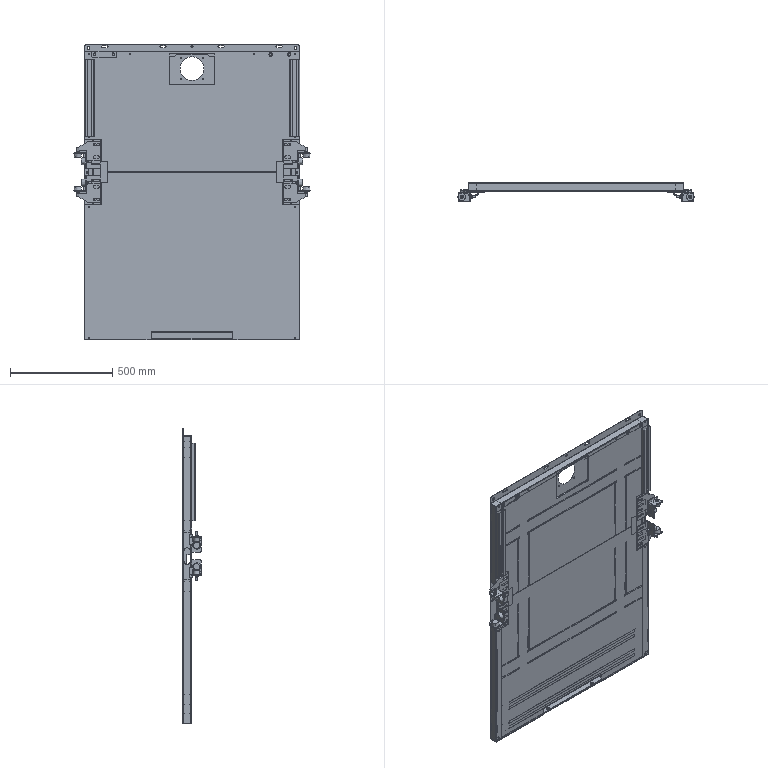Part | SolidWorks | features ReferencePattern 8, MirrorCompFeat 5 | 58 solids | 2126 faces | box 1154 x 89.5 x 1445 mm | volume 6635667 mm3 | plane 1428 | cylinder 578 | cone 120 | commonest cylinder face diameters 10 x112 0.4 x74 11 x52 3.4 x48 20 x42 9 x32